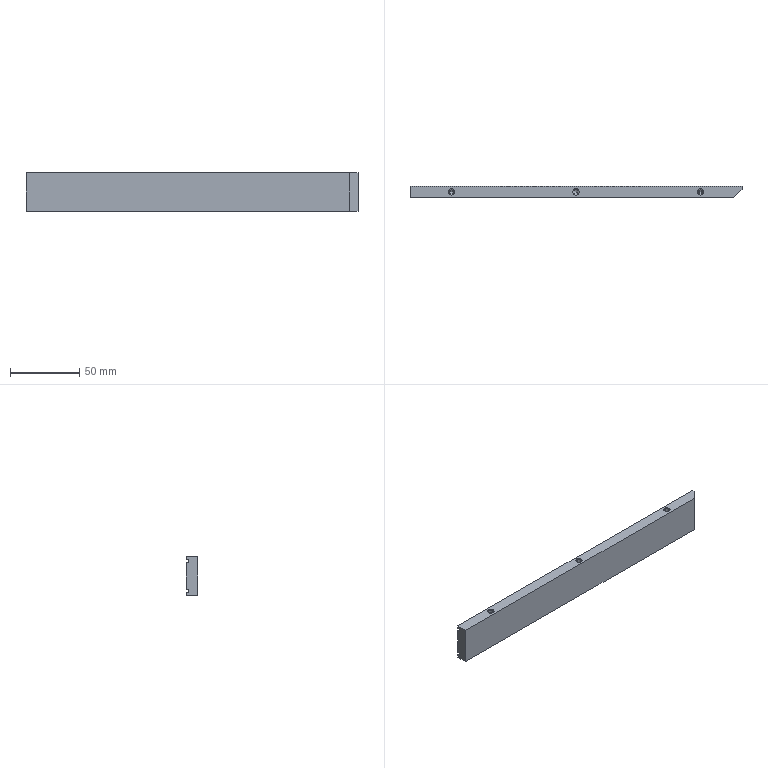Part | NX | 1 solid | 63 faces | box 240 x 8 x 27.6 mm | volume 50259 mm3 | cylinder 24 | cone 24 | plane 15 | commonest cylinder face diameters 3.3 x24